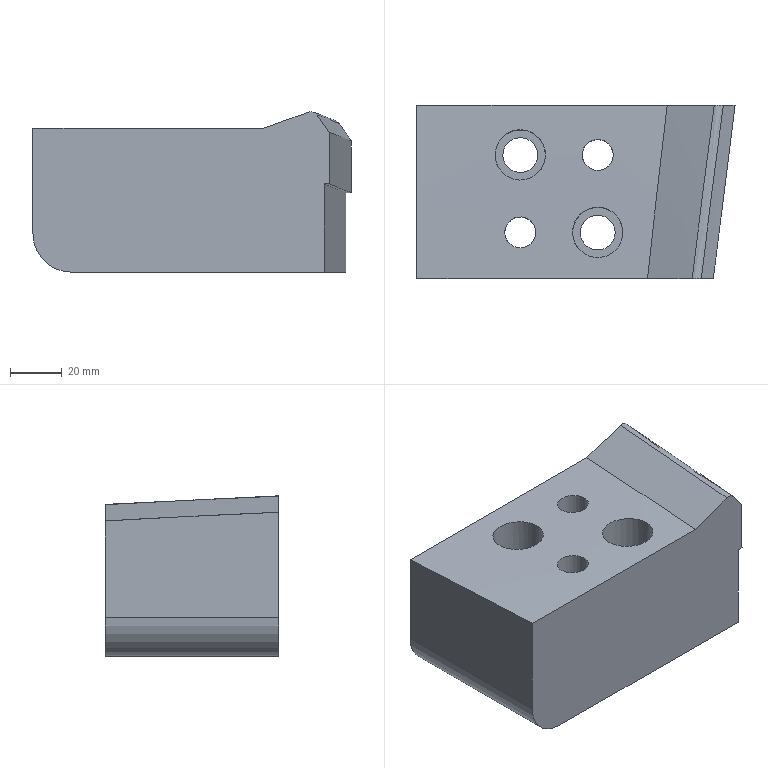Part | NX | features MAIN_BODY 2 | 1 solid | 20 faces | box 123.132 x 67 x 62.076 mm | volume 387142 mm3 | spline 7 | cylinder 7 | plane 6 | commonest cylinder face diameters 12 x2 13.5 x2 19.5 x2 30 x1
STEP:
#1=CARTESIAN_POINT('',(-841.75,399.358,-90.));
#2=VERTEX_POINT('',#1);
#3=CARTESIAN_POINT('',(-835.,399.358,-90.));
#4=DIRECTION('',(-0.000000341,-0.00000017,-1.));
#5=DIRECTION('',(-1.,0.,0.000000341));
#6=AXIS2_PLACEMENT_3D('',#3,#4,#5);
#7=CIRCLE('',#6,6.75);
#8=EDGE_CURVE('',#2,#2,#7,.F.);
#9=ORIENTED_EDGE('',*,*,#8,.T.);
#10=EDGE_LOOP('',(#9));
#11=FACE_BOUND('',#10,.T.);
#12=CARTESIAN_POINT('',(-841.,369.358,-90.));
#13=VERTEX_POINT('',#12);
#14=CARTESIAN_POINT('',(-835.,369.358,-90.));
#15=DIRECTION('',(-0.000000341,-0.00000017,-1.));
#16=DIRECTION('',(-1.,0.,0.000000341));
#17=AXIS2_PLACEMENT_3D('',#14,#15,#16);
#18=CIRCLE('',#17,6.);
#19=EDGE_CURVE('',#13,#13,#18,.F.);
#20=ORIENTED_EDGE('',*,*,#19,.T.);
#21=EDGE_LOOP('',(#20));
#22=FACE_BOUND('',#21,.T.);
#23=CARTESIAN_POINT('',(-811.75,369.358,-90.));
#24=VERTEX_POINT('',#23);
#25=CARTESIAN_POINT('',(-805.,369.358,-90.));
#26=DIRECTION('',(-0.000000341,-0.00000017,-1.));
#27=DIRECTION('',(-1.,0.,0.000000341));
#28=AXIS2_PLACEMENT_3D('',#25,#26,#27);
#29=CIRCLE('',#28,6.75);
#30=EDGE_CURVE('',#24,#24,#29,.F.);
#31=ORIENTED_EDGE('',*,*,#30,.T.);
#32=EDGE_LOOP('',(#31));
#33=FACE_BOUND('',#32,.T.);
#34=CARTESIAN_POINT('',(-811.,399.358,-90.));
#35=VERTEX_POINT('',#34);
#36=CARTESIAN_POINT('',(-805.,399.358,-90.));
#37=DIRECTION('',(-0.000000341,-0.00000017,-1.));
#38=DIRECTION('',(-1.,0.,0.000000341));
#39=AXIS2_PLACEMENT_3D('',#36,#37,#38);
#40=CIRCLE('',#39,6.);
#41=EDGE_CURVE('',#35,#35,#40,.F.);
#42=ORIENTED_EDGE('',*,*,#41,.T.);
#43=EDGE_LOOP('',(#42));
#44=FACE_BOUND('',#43,.T.);
#45=CARTESIAN_POINT('',(-860.,351.533,-90.));
#46=VERTEX_POINT('',#45);
#47=CARTESIAN_POINT('',(-762.297,351.533,-90.));
#48=VERTEX_POINT('',#47);
#49=CARTESIAN_POINT('',(-780.,351.533,-90.));
#50=DIRECTION('',(1.,0.000000011,-0.000000341));
#51=VECTOR('',#50,1000.);
#52=LINE('',#49,#51);
#53=EDGE_CURVE('',#46,#48,#52,.T.);
#54=ORIENTED_EDGE('',*,*,#53,.F.);
#55=CARTESIAN_POINT('',(-860.,418.533,-90.));
#56=VERTEX_POINT('',#55);
#57=CARTESIAN_POINT('',(-860.,1058.533,-90.));
#58=DIRECTION('',(-0.000000011,1.,-0.00000017));
#59=VECTOR('',#58,1000.);
#60=LINE('',#57,#59);
#61=EDGE_CURVE('',#46,#56,#60,.T.);
#62=ORIENTED_EDGE('',*,*,#61,.T.);
#63=CARTESIAN_POINT('',(-753.885,418.533,-90.));
#64=VERTEX_POINT('',#63);
#65=CARTESIAN_POINT('',(-780.,418.533,-90.));
#66=DIRECTION('',(1.,0.000000011,-0.000000341));
#67=VECTOR('',#66,1000.);
#68=LINE('',#65,#67);
#69=EDGE_CURVE('',#56,#64,#68,.T.);
#70=ORIENTED_EDGE('',*,*,#69,.T.);
#71=CARTESIAN_POINT('',(-753.885,418.533,-90.));
#72=CARTESIAN_POINT('',(-755.339,407.373,-90.));
#73=CARTESIAN_POINT('',(-758.303,385.059,-90.));
#74=CARTESIAN_POINT('',(-760.967,362.708,-90.));
#75=CARTESIAN_POINT('',(-762.297,351.533,-90.));
#76=B_SPLINE_CURVE_WITH_KNOTS('',3,(#71,#72,#73,#74,#75),.UNSPECIFIED.,.F.,.F.,(4,1,4),(0.,0.03376,0.06753),.UNSPECIFIED.);
#77=EDGE_CURVE('',#64,#48,#76,.T.);
#78=ORIENTED_EDGE('',*,*,#77,.T.);
#79=EDGE_LOOP('',(#54,#62,#70,#78));
#80=FACE_BOUND('',#79,.T.);
#81=CARTESIAN_POINT('',(-780.,1058.533,-90.));
#82=DIRECTION('',(-0.000000341,-0.00000017,-1.));
#83=DIRECTION('',(-0.000000011,1.,-0.00000017));
#84=AXIS2_PLACEMENT_3D('',#81,#82,#83);
#85=PLANE('',#84);
#86=ADVANCED_FACE('',(#11,#22,#33,#44,#80),#85,.T.);
#87=CARTESIAN_POINT('',(-751.868,418.533,-39.201));
#88=VERTEX_POINT('',#87);
#89=CARTESIAN_POINT('',(-756.435,418.533,-32.553));
#90=VERTEX_POINT('',#89);
#91=CARTESIAN_POINT('',(-751.868,418.533,-39.201));
#92=CARTESIAN_POINT('',(-753.39,418.533,-36.985));
#93=CARTESIAN_POINT('',(-754.912,418.533,-34.769));
#94=CARTESIAN_POINT('',(-756.435,418.533,-32.553));
#95=B_SPLINE_CURVE_WITH_KNOTS('',3,(#91,#92,#93,#94),.UNSPECIFIED.,.F.,.F.,(4,4),(0.,0.008065),.UNSPECIFIED.);
#96=EDGE_CURVE('',#88,#90,#95,.T.);
#97=ORIENTED_EDGE('',*,*,#96,.F.);
#98=CARTESIAN_POINT('',(-751.868,418.533,-59.201));
#99=VERTEX_POINT('',#98);
#100=CARTESIAN_POINT('',(-751.868,418.533,-39.201));
#101=CARTESIAN_POINT('',(-751.868,418.533,-45.868));
#102=CARTESIAN_POINT('',(-751.868,418.533,-52.535));
#103=CARTESIAN_POINT('',(-751.868,418.533,-59.201));
#104=B_SPLINE_CURVE_WITH_KNOTS('',3,(#100,#101,#102,#103),.UNSPECIFIED.,.F.,.F.,(4,4),(0.01625,0.03625),.UNSPECIFIED.);
#105=EDGE_CURVE('',#88,#99,#104,.T.);
#106=ORIENTED_EDGE('',*,*,#105,.T.);
#107=CARTESIAN_POINT('',(-753.885,418.533,-59.187));
#108=VERTEX_POINT('',#107);
#109=CARTESIAN_POINT('',(-753.885,418.533,-59.187));
#110=CARTESIAN_POINT('',(-753.213,418.533,-59.192));
#111=CARTESIAN_POINT('',(-752.541,418.533,-59.197));
#112=CARTESIAN_POINT('',(-751.868,418.533,-59.201));
#113=B_SPLINE_CURVE_WITH_KNOTS('',3,(#109,#110,#111,#112),.UNSPECIFIED.,.F.,.F.,(4,4),(0.,0.002017),.UNSPECIFIED.);
#114=EDGE_CURVE('',#108,#99,#113,.T.);
#115=ORIENTED_EDGE('',*,*,#114,.F.);
#116=CARTESIAN_POINT('',(-753.885,418.533,-59.187));
#117=CARTESIAN_POINT('',(-753.885,418.533,-69.458));
#118=CARTESIAN_POINT('',(-753.885,418.533,-79.729));
#119=CARTESIAN_POINT('',(-753.885,418.533,-90.));
#120=B_SPLINE_CURVE_WITH_KNOTS('',3,(#116,#117,#118,#119),.UNSPECIFIED.,.F.,.F.,(4,4),(-0.004527,0.02629),.UNSPECIFIED.);
#121=EDGE_CURVE('',#108,#64,#120,.T.);
#122=ORIENTED_EDGE('',*,*,#121,.T.);
#123=ORIENTED_EDGE('',*,*,#69,.F.);
#124=CARTESIAN_POINT('',(-875.,418.533,-75.));
#125=VERTEX_POINT('',#124);
#126=CARTESIAN_POINT('',(-860.,418.533,-75.));
#127=DIRECTION('',(-0.000000011,1.,-0.00000017));
#128=DIRECTION('',(0.,0.00000017,1.));
#129=AXIS2_PLACEMENT_3D('',#126,#127,#128);
#130=CIRCLE('',#129,15.);
#131=EDGE_CURVE('',#56,#125,#130,.T.);
#132=ORIENTED_EDGE('',*,*,#131,.T.);
#133=CARTESIAN_POINT('',(-875.,418.533,-37.652));
#134=VERTEX_POINT('',#133);
#135=CARTESIAN_POINT('',(-875.,418.533,-90.));
#136=DIRECTION('',(-0.000000341,-0.00000017,-1.));
#137=VECTOR('',#136,1000.);
#138=LINE('',#135,#137);
#139=EDGE_CURVE('',#125,#134,#138,.F.);
#140=ORIENTED_EDGE('',*,*,#139,.T.);
#141=CARTESIAN_POINT('',(-778.148,418.533,-37.652));
#142=VERTEX_POINT('',#141);
#143=CARTESIAN_POINT('',(-820.117,418.533,-37.652));
#144=DIRECTION('',(1.,0.000000011,-0.000000341));
#145=VECTOR('',#144,1000.);
#146=LINE('',#143,#145);
#147=EDGE_CURVE('',#134,#142,#146,.T.);
#148=ORIENTED_EDGE('',*,*,#147,.T.);
#149=CARTESIAN_POINT('',(-759.941,418.533,-31.393));
#150=VERTEX_POINT('',#149);
#151=CARTESIAN_POINT('',(-759.941,418.533,-31.393));
#152=CARTESIAN_POINT('',(-766.01,418.533,-33.479));
#153=CARTESIAN_POINT('',(-772.079,418.533,-35.565));
#154=CARTESIAN_POINT('',(-778.148,418.533,-37.652));
#155=B_SPLINE_CURVE_WITH_KNOTS('',3,(#151,#152,#153,#154),.UNSPECIFIED.,.F.,.F.,(4,4),(0.02556,0.04482),.UNSPECIFIED.);
#156=EDGE_CURVE('',#150,#142,#155,.T.);
#157=ORIENTED_EDGE('',*,*,#156,.F.);
#158=CARTESIAN_POINT('',(-756.435,418.533,-32.553));
#159=CARTESIAN_POINT('',(-757.19,418.533,-31.454));
#160=CARTESIAN_POINT('',(-758.679,418.533,-30.959));
#161=CARTESIAN_POINT('',(-759.941,418.533,-31.393));
#162=B_SPLINE_CURVE_WITH_KNOTS('',3,(#158,#159,#160,#161),.UNSPECIFIED.,.F.,.F.,(4,4),(0.,0.003944),.UNSPECIFIED.);
#163=EDGE_CURVE('',#90,#150,#162,.T.);
#164=ORIENTED_EDGE('',*,*,#163,.F.);
#165=EDGE_LOOP('',(#97,#106,#115,#122,#123,#132,#140,#148,#157,#164));
#166=FACE_BOUND('',#165,.T.);
#167=CARTESIAN_POINT('',(-840.,418.533,-90.));
#168=DIRECTION('',(-0.000000011,1.,-0.00000017));
#169=DIRECTION('',(0.000000341,0.00000017,1.));
#170=AXIS2_PLACEMENT_3D('',#167,#168,#169);
#171=PLANE('',#170);
#172=ADVANCED_FACE('',(#166),#171,.T.);
#173=CARTESIAN_POINT('',(-760.283,351.533,-35.819));
#174=VERTEX_POINT('',#173);
#175=CARTESIAN_POINT('',(-760.283,351.533,-55.819));
#176=VERTEX_POINT('',#175);
#177=CARTESIAN_POINT('',(-760.283,351.533,-35.819));
#178=CARTESIAN_POINT('',(-760.283,351.533,-42.486));
#179=CARTESIAN_POINT('',(-760.283,351.533,-49.152));
#180=CARTESIAN_POINT('',(-760.283,351.533,-55.819));
#181=B_SPLINE_CURVE_WITH_KNOTS('',3,(#177,#178,#179,#180),.UNSPECIFIED.,.F.,.F.,(4,4),(0.009058,0.02906),.UNSPECIFIED.);
#182=EDGE_CURVE('',#174,#176,#181,.T.);
#183=ORIENTED_EDGE('',*,*,#182,.T.);
#184=CARTESIAN_POINT('',(-751.868,418.533,-59.201));
#185=CARTESIAN_POINT('',(-753.322,407.375,-58.596));
#186=CARTESIAN_POINT('',(-756.286,385.067,-57.354));
#187=CARTESIAN_POINT('',(-758.953,362.711,-56.325));
#188=CARTESIAN_POINT('',(-760.283,351.533,-55.819));
#189=B_SPLINE_CURVE_WITH_KNOTS('',3,(#184,#185,#186,#187,#188),.UNSPECIFIED.,.F.,.F.,(4,1,4),(0.,0.03381,0.06761),.UNSPECIFIED.);
#190=EDGE_CURVE('',#99,#176,#189,.T.);
#191=ORIENTED_EDGE('',*,*,#190,.F.);
#192=ORIENTED_EDGE('',*,*,#105,.F.);
#193=CARTESIAN_POINT('',(-760.283,351.533,-35.819));
#194=CARTESIAN_POINT('',(-758.953,362.711,-36.325));
#195=CARTESIAN_POINT('',(-756.286,385.067,-37.354));
#196=CARTESIAN_POINT('',(-753.322,407.375,-38.596));
#197=CARTESIAN_POINT('',(-751.868,418.533,-39.201));
#198=B_SPLINE_CURVE_WITH_KNOTS('',3,(#193,#194,#195,#196,#197),.UNSPECIFIED.,.F.,.F.,(4,1,4),(0.,0.03381,0.06761),.UNSPECIFIED.);
#199=EDGE_CURVE('',#174,#88,#198,.T.);
#200=ORIENTED_EDGE('',*,*,#199,.F.);
#201=EDGE_LOOP('',(#183,#191,#192,#200));
#202=FACE_BOUND('',#201,.T.);
#203=CARTESIAN_POINT('',(-760.331,351.13,-55.941));
#204=CARTESIAN_POINT('',(-760.331,351.13,-35.657));
#205=CARTESIAN_POINT('',(-758.993,362.375,-56.467));
#206=CARTESIAN_POINT('',(-758.993,362.375,-36.183));
#207=CARTESIAN_POINT('',(-756.313,384.864,-57.522));
#208=CARTESIAN_POINT('',(-756.313,384.864,-37.238));
#209=CARTESIAN_POINT('',(-753.331,407.307,-58.731));
#210=CARTESIAN_POINT('',(-753.331,407.307,-38.447));
#211=CARTESIAN_POINT('',(-751.868,418.533,-59.322));
#212=CARTESIAN_POINT('',(-751.868,418.533,-39.037));
#213=B_SPLINE_SURFACE_WITH_KNOTS('',3,1,((#203,#204),(#205,#206),(#207,#208),(#209,#210),(#211,#212)),.SURF_OF_LINEAR_EXTRUSION.,.F.,.F.,.F.,(4,1,4),(2,2),(-0.3914,0.6746,1.741),(0.,1.),.UNSPECIFIED.);
#214=ADVANCED_FACE('',(#202),#213,.T.);
#215=ORIENTED_EDGE('',*,*,#139,.F.);
#216=CARTESIAN_POINT('',(-875.,351.533,-75.));
#217=VERTEX_POINT('',#216);
#218=CARTESIAN_POINT('',(-875.,739.25,-75.));
#219=DIRECTION('',(0.000000011,-1.,0.00000017));
#220=VECTOR('',#219,1000.);
#221=LINE('',#218,#220);
#222=EDGE_CURVE('',#125,#217,#221,.T.);
#223=ORIENTED_EDGE('',*,*,#222,.T.);
#224=CARTESIAN_POINT('',(-875.,351.533,-34.317));
#225=VERTEX_POINT('',#224);
#226=CARTESIAN_POINT('',(-875.,351.533,-90.));
#227=DIRECTION('',(-0.000000341,-0.00000017,-1.));
#228=VECTOR('',#227,1000.);
#229=LINE('',#226,#228);
#230=EDGE_CURVE('',#217,#225,#229,.F.);
#231=ORIENTED_EDGE('',*,*,#230,.T.);
#232=CARTESIAN_POINT('',(-875.,351.533,-34.317));
#233=CARTESIAN_POINT('',(-875.,373.874,-35.265));
#234=CARTESIAN_POINT('',(-875.,396.208,-36.367));
#235=CARTESIAN_POINT('',(-875.,418.533,-37.652));
#236=B_SPLINE_CURVE_WITH_KNOTS('',3,(#232,#233,#234,#235),.UNSPECIFIED.,.F.,.F.,(4,4),(0.277,0.3441),.UNSPECIFIED.);
#237=EDGE_CURVE('',#134,#225,#236,.F.);
#238=ORIENTED_EDGE('',*,*,#237,.F.);
#239=EDGE_LOOP('',(#215,#223,#231,#238));
#240=FACE_BOUND('',#239,.T.);
#241=CARTESIAN_POINT('',(-875.,739.25,-90.));
#242=DIRECTION('',(-1.,-0.000000011,0.000000341));
#243=DIRECTION('',(-0.000000341,-0.00000017,-1.));
#244=AXIS2_PLACEMENT_3D('',#241,#242,#243);
#245=PLANE('',#244);
#246=ADVANCED_FACE('',(#240),#245,.T.);
#247=CARTESIAN_POINT('',(-802.615,378.812,-35.56));
#248=VERTEX_POINT('',#247);
#249=CARTESIAN_POINT('',(-810.554,378.63,-35.551));
#250=CARTESIAN_POINT('',(-802.353,379.838,-35.61));
#251=CARTESIAN_POINT('',(-795.722,374.891,-35.371));
#252=CARTESIAN_POINT('',(-794.523,366.727,-34.987));
#253=CARTESIAN_POINT('',(-799.45,360.085,-34.688));
#254=CARTESIAN_POINT('',(-807.643,358.881,-34.635));
#255=CARTESIAN_POINT('',(-814.27,363.813,-34.854));
#256=CARTESIAN_POINT('',(-815.479,371.987,-35.232));
#257=CARTESIAN_POINT('',(-810.554,378.63,-35.551));
#258=CARTESIAN_POINT('',(-802.353,379.838,-35.61));
#259=CARTESIAN_POINT('',(-795.722,374.891,-35.371));
#260=B_SPLINE_CURVE_WITH_KNOTS('',3,(#249,#250,#251,#252,#253,#254,#255,#256,#257,#258,#259),.UNSPECIFIED.,.T.,.F.,(1,1,1,1,1,1,1,1,1,1,1,1,1,1,1),(-0.02287,-0.01525,-0.007624,0.,0.007624,0.01525,0.02287,0.0305,0.03812,0.04574,0.05337,0.06099,0.06862,0.07624,0.08386),.UNSPECIFIED.);
#261=EDGE_CURVE('',#248,#248,#260,.T.);
#262=ORIENTED_EDGE('',*,*,#261,.T.);
#263=EDGE_LOOP('',(#262));
#264=FACE_BOUND('',#263,.T.);
#265=CARTESIAN_POINT('',(-806.104,405.256,-36.91));
#266=VERTEX_POINT('',#265);
#267=CARTESIAN_POINT('',(-810.492,403.108,-36.793));
#268=CARTESIAN_POINT('',(-806.223,405.897,-36.944));
#269=CARTESIAN_POINT('',(-801.239,404.841,-36.887));
#270=CARTESIAN_POINT('',(-798.467,400.584,-36.658));
#271=CARTESIAN_POINT('',(-799.51,395.607,-36.398));
#272=CARTESIAN_POINT('',(-803.775,392.823,-36.256));
#273=CARTESIAN_POINT('',(-808.753,393.871,-36.309));
#274=CARTESIAN_POINT('',(-811.534,398.131,-36.529));
#275=CARTESIAN_POINT('',(-810.492,403.108,-36.793));
#276=CARTESIAN_POINT('',(-806.223,405.897,-36.944));
#277=CARTESIAN_POINT('',(-801.239,404.841,-36.887));
#278=B_SPLINE_CURVE_WITH_KNOTS('',3,(#267,#268,#269,#270,#271,#272,#273,#274,#275,#276,#277),.UNSPECIFIED.,.T.,.F.,(1,1,1,1,1,1,1,1,1,1,1,1,1,1,1),(-0.01408,-0.009385,-0.004692,0.,0.004692,0.009385,0.01408,0.01877,0.02346,0.02815,0.03285,0.03754,0.04223,0.04692,0.05162),.UNSPECIFIED.);
#279=EDGE_CURVE('',#266,#266,#278,.T.);
#280=ORIENTED_EDGE('',*,*,#279,.T.);
#281=EDGE_LOOP('',(#280));
#282=FACE_BOUND('',#281,.T.);
#283=CARTESIAN_POINT('',(-785.768,351.533,-34.317));
#284=VERTEX_POINT('',#283);
#285=CARTESIAN_POINT('',(-823.992,351.533,-34.317));
#286=DIRECTION('',(1.,0.000000011,-0.000000341));
#287=VECTOR('',#286,1000.);
#288=LINE('',#285,#287);
#289=EDGE_CURVE('',#225,#284,#288,.T.);
#290=ORIENTED_EDGE('',*,*,#289,.T.);
#291=CARTESIAN_POINT('',(-778.148,418.533,-37.652));
#292=CARTESIAN_POINT('',(-780.817,396.223,-36.368));
#293=CARTESIAN_POINT('',(-783.364,373.889,-35.266));
#294=CARTESIAN_POINT('',(-785.768,351.533,-34.317));
#295=B_SPLINE_CURVE_WITH_KNOTS('',3,(#291,#292,#293,#294),.UNSPECIFIED.,.F.,.F.,(4,4),(0.1671,0.2344),.UNSPECIFIED.);
#296=EDGE_CURVE('',#142,#284,#295,.T.);
#297=ORIENTED_EDGE('',*,*,#296,.F.);
#298=ORIENTED_EDGE('',*,*,#147,.F.);
#299=ORIENTED_EDGE('',*,*,#237,.T.);
#300=EDGE_LOOP('',(#290,#297,#298,#299));
#301=FACE_BOUND('',#300,.T.);
#302=CARTESIAN_POINT('',(-837.117,374.973,-35.376));
#303=VERTEX_POINT('',#302);
#304=CARTESIAN_POINT('',(-841.061,372.092,-35.239));
#305=CARTESIAN_POINT('',(-837.346,375.582,-35.405));
#306=CARTESIAN_POINT('',(-832.255,375.414,-35.397));
#307=CARTESIAN_POINT('',(-828.781,371.706,-35.22));
#308=CARTESIAN_POINT('',(-828.94,366.622,-34.983));
#309=CARTESIAN_POINT('',(-832.652,363.137,-34.825));
#310=CARTESIAN_POINT('',(-837.736,363.299,-34.832));
#311=CARTESIAN_POINT('',(-841.22,367.009,-35.001));
#312=CARTESIAN_POINT('',(-841.061,372.092,-35.239));
#313=CARTESIAN_POINT('',(-837.346,375.582,-35.405));
#314=CARTESIAN_POINT('',(-832.255,375.414,-35.397));
#315=B_SPLINE_CURVE_WITH_KNOTS('',3,(#304,#305,#306,#307,#308,#309,#310,#311,#312,#313,#314),.UNSPECIFIED.,.T.,.F.,(1,1,1,1,1,1,1,1,1,1,1,1,1,1,1),(-0.01408,-0.009384,-0.004692,0.,0.004692,0.009384,0.01408,0.01877,0.02346,0.02815,0.03284,0.03753,0.04223,0.04692,0.05161),.UNSPECIFIED.);
#316=EDGE_CURVE('',#303,#303,#315,.T.);
#317=ORIENTED_EDGE('',*,*,#316,.T.);
#318=EDGE_LOOP('',(#317));
#319=FACE_BOUND('',#318,.T.);
#320=CARTESIAN_POINT('',(-844.701,400.333,-36.646));
#321=VERTEX_POINT('',#320);
#322=CARTESIAN_POINT('',(-843.364,392.516,-36.238));
#323=CARTESIAN_POINT('',(-845.751,400.44,-36.648));
#324=CARTESIAN_POINT('',(-841.839,407.721,-37.043));
#325=CARTESIAN_POINT('',(-833.927,410.11,-37.176));
#326=CARTESIAN_POINT('',(-826.634,406.198,-36.959));
#327=CARTESIAN_POINT('',(-824.252,398.282,-36.535));
#328=CARTESIAN_POINT('',(-828.148,391.005,-36.162));
#329=CARTESIAN_POINT('',(-836.069,388.604,-36.043));
#330=CARTESIAN_POINT('',(-843.364,392.516,-36.238));
#331=CARTESIAN_POINT('',(-845.751,400.44,-36.648));
#332=CARTESIAN_POINT('',(-841.839,407.721,-37.043));
#333=B_SPLINE_CURVE_WITH_KNOTS('',3,(#322,#323,#324,#325,#326,#327,#328,#329,#330,#331,#332),.UNSPECIFIED.,.T.,.F.,(1,1,1,1,1,1,1,1,1,1,1,1,1,1,1),(-0.02288,-0.01525,-0.007625,0.,0.007625,0.01525,0.02288,0.0305,0.03813,0.04575,0.05338,0.061,0.06863,0.07625,0.08388),.UNSPECIFIED.);
#334=EDGE_CURVE('',#321,#321,#333,.T.);
#335=ORIENTED_EDGE('',*,*,#334,.T.);
#336=EDGE_LOOP('',(#335));
#337=FACE_BOUND('',#336,.T.);
#338=CARTESIAN_POINT('',(-875.586,418.533,-37.652));
#339=CARTESIAN_POINT('',(-776.779,418.533,-37.652));
#340=CARTESIAN_POINT('',(-877.041,407.36,-37.009));
#341=CARTESIAN_POINT('',(-778.234,407.36,-37.009));
#342=CARTESIAN_POINT('',(-880.005,385.084,-35.832));
#343=CARTESIAN_POINT('',(-781.198,385.084,-35.832));
#344=CARTESIAN_POINT('',(-882.657,362.711,-34.791));
#345=CARTESIAN_POINT('',(-783.85,362.711,-34.791));
#346=CARTESIAN_POINT('',(-883.99,351.533,-34.317));
#347=CARTESIAN_POINT('',(-785.183,351.533,-34.317));
#348=B_SPLINE_SURFACE_WITH_KNOTS('',3,1,((#338,#339),(#340,#341),(#342,#343),(#344,#345),(#346,#347)),.SURF_OF_LINEAR_EXTRUSION.,.F.,.F.,.F.,(4,1,4),(2,2),(-0.00601,0.4948,0.9956),(0.,1.),.UNSPECIFIED.);
#349=ADVANCED_FACE('',(#264,#282,#301,#319,#337),#348,.T.);
#350=CARTESIAN_POINT('',(-768.455,351.533,-28.093));
#351=VERTEX_POINT('',#350);
#352=CARTESIAN_POINT('',(-785.768,351.533,-34.317));
#353=CARTESIAN_POINT('',(-779.997,351.533,-32.242));
#354=CARTESIAN_POINT('',(-774.226,351.533,-30.167));
#355=CARTESIAN_POINT('',(-768.455,351.533,-28.093));
#356=B_SPLINE_CURVE_WITH_KNOTS('',3,(#352,#353,#354,#355),.UNSPECIFIED.,.F.,.F.,(4,4),(0.07252,0.09092),.UNSPECIFIED.);
#357=EDGE_CURVE('',#351,#284,#356,.F.);
#358=ORIENTED_EDGE('',*,*,#357,.T.);
#359=ORIENTED_EDGE('',*,*,#289,.F.);
#360=ORIENTED_EDGE('',*,*,#230,.F.);
#361=CARTESIAN_POINT('',(-860.,351.533,-75.));
#362=DIRECTION('',(-0.000000011,1.,-0.00000017));
#363=DIRECTION('',(0.,0.00000017,1.));
#364=AXIS2_PLACEMENT_3D('',#361,#362,#363);
#365=CIRCLE('',#364,15.);
#366=EDGE_CURVE('',#217,#46,#365,.F.);
#367=ORIENTED_EDGE('',*,*,#366,.T.);
#368=ORIENTED_EDGE('',*,*,#53,.T.);
#369=CARTESIAN_POINT('',(-762.297,351.533,-55.808));
#370=VERTEX_POINT('',#369);
#371=CARTESIAN_POINT('',(-762.297,351.533,-55.808));
#372=CARTESIAN_POINT('',(-762.297,351.533,-67.206));
#373=CARTESIAN_POINT('',(-762.297,351.533,-78.603));
#374=CARTESIAN_POINT('',(-762.297,351.533,-90.));
#375=B_SPLINE_CURVE_WITH_KNOTS('',3,(#371,#372,#373,#374),.UNSPECIFIED.,.F.,.F.,(4,4),(-0.01041,0.02379),.UNSPECIFIED.);
#376=EDGE_CURVE('',#370,#48,#375,.T.);
#377=ORIENTED_EDGE('',*,*,#376,.F.);
#378=CARTESIAN_POINT('',(-760.283,351.533,-55.819));
#379=CARTESIAN_POINT('',(-760.955,351.533,-55.816));
#380=CARTESIAN_POINT('',(-761.626,351.533,-55.812));
#381=CARTESIAN_POINT('',(-762.297,351.533,-55.808));
#382=B_SPLINE_CURVE_WITH_KNOTS('',3,(#378,#379,#380,#381),.UNSPECIFIED.,.F.,.F.,(4,4),(0.,0.002014),.UNSPECIFIED.);
#383=EDGE_CURVE('',#176,#370,#382,.T.);
#384=ORIENTED_EDGE('',*,*,#383,.F.);
#385=ORIENTED_EDGE('',*,*,#182,.F.);
#386=CARTESIAN_POINT('',(-764.943,351.533,-29.203));
#387=VERTEX_POINT('',#386);
#388=CARTESIAN_POINT('',(-764.943,351.533,-29.203));
#389=CARTESIAN_POINT('',(-763.39,351.533,-31.408));
#390=CARTESIAN_POINT('',(-761.836,351.533,-33.614));
#391=CARTESIAN_POINT('',(-760.283,351.533,-35.819));
#392=B_SPLINE_CURVE_WITH_KNOTS('',3,(#388,#389,#390,#391),.UNSPECIFIED.,.F.,.F.,(4,4),(0.007518,0.01561),.UNSPECIFIED.);
#393=EDGE_CURVE('',#387,#174,#392,.T.);
#394=ORIENTED_EDGE('',*,*,#393,.F.);
#395=CARTESIAN_POINT('',(-768.455,351.533,-28.093));
#396=CARTESIAN_POINT('',(-767.203,351.533,-27.643));
#397=CARTESIAN_POINT('',(-765.71,351.533,-28.115));
#398=CARTESIAN_POINT('',(-764.943,351.533,-29.203));
#399=B_SPLINE_CURVE_WITH_KNOTS('',3,(#395,#396,#397,#398),.UNSPECIFIED.,.F.,.F.,(4,4),(0.,0.003935),.UNSPECIFIED.);
#400=EDGE_CURVE('',#351,#387,#399,.T.);
#401=ORIENTED_EDGE('',*,*,#400,.F.);
#402=EDGE_LOOP('',(#358,#359,#360,#367,#368,#377,#384,#385,#394,#401));
#403=FACE_BOUND('',#402,.T.);
#404=CARTESIAN_POINT('',(-840.,351.533,-90.));
#405=DIRECTION('',(-0.000000011,1.,-0.00000017));
#406=DIRECTION('',(0.000000341,0.00000017,1.));
#407=AXIS2_PLACEMENT_3D('',#404,#405,#406);
#408=PLANE('',#407);
#409=ADVANCED_FACE('',(#403),#408,.F.);
#410=CARTESIAN_POINT('',(-844.75,399.358,-80.));
#411=VERTEX_POINT('',#410);
#412=CARTESIAN_POINT('',(-835.,399.358,-80.));
#413=DIRECTION('',(-0.000000341,-0.00000017,-1.));
#414=DIRECTION('',(-1.,0.,0.000000341));
#415=AXIS2_PLACEMENT_3D('',#412,#413,#414);
#416=CIRCLE('',#415,9.75);
#417=EDGE_CURVE('',#411,#411,#416,.F.);
#418=ORIENTED_EDGE('',*,*,#417,.F.);
#419=EDGE_LOOP('',(#418));
#420=FACE_BOUND('',#419,.T.);
#421=ORIENTED_EDGE('',*,*,#334,.F.);
#422=EDGE_LOOP('',(#421));
#423=FACE_BOUND('',#422,.T.);
#424=CARTESIAN_POINT('',(-835.,399.358,-70.));
#425=DIRECTION('',(0.000000341,0.00000017,1.));
#426=DIRECTION('',(0.000000011,-1.,0.00000017));
#427=AXIS2_PLACEMENT_3D('',#424,#425,#426);
#428=CYLINDRICAL_SURFACE('',#427,9.75);
#429=ADVANCED_FACE('',(#420,#423),#428,.F.);
#430=CARTESIAN_POINT('',(-841.75,399.358,-80.));
#431=VERTEX_POINT('',#430);
#432=CARTESIAN_POINT('',(-835.,399.358,-80.));
#433=DIRECTION('',(-0.000000341,-0.00000017,-1.));
#434=DIRECTION('',(-1.,0.,0.000000341));
#435=AXIS2_PLACEMENT_3D('',#432,#433,#434);
#436=CIRCLE('',#435,6.75);
#437=EDGE_CURVE('',#431,#431,#436,.F.);
#438=ORIENTED_EDGE('',*,*,#437,.T.);
#439=EDGE_LOOP('',(#438));
#440=FACE_BOUND('',#439,.T.);
#441=ORIENTED_EDGE('',*,*,#8,.F.);
#442=EDGE_LOOP('',(#441));
#443=FACE_BOUND('',#442,.T.);
#444=CARTESIAN_POINT('',(-835.,399.358,-90.));
#445=DIRECTION('',(0.000000341,0.00000017,1.));
#446=DIRECTION('',(0.000000011,-1.,0.00000017));
#447=AXIS2_PLACEMENT_3D('',#444,#445,#446);
#448=CYLINDRICAL_SURFACE('',#447,6.75);
#449=ADVANCED_FACE('',(#440,#443),#448,.F.);
#450=ORIENTED_EDGE('',*,*,#437,.F.);
#451=EDGE_LOOP('',(#450));
#452=FACE_BOUND('',#451,.T.);
#453=ORIENTED_EDGE('',*,*,#417,.T.);
#454=EDGE_LOOP('',(#453));
#455=FACE_BOUND('',#454,.T.);
#456=CARTESIAN_POINT('',(-835.,399.358,-80.));
#457=DIRECTION('',(-0.000000341,-0.00000017,-1.));
#458=DIRECTION('',(-0.000000011,1.,-0.00000017));
#459=AXIS2_PLACEMENT_3D('',#456,#457,#458);
#460=PLANE('',#459);
#461=ADVANCED_FACE('',(#452,#455),#460,.F.);
#462=ORIENTED_EDGE('',*,*,#19,.F.);
#463=EDGE_LOOP('',(#462));
#464=FACE_BOUND('',#463,.T.);
#465=ORIENTED_EDGE('',*,*,#316,.F.);
#466=EDGE_LOOP('',(#465));
#467=FACE_BOUND('',#466,.T.);
#468=CARTESIAN_POINT('',(-835.,369.358,-90.));
#469=DIRECTION('',(0.000000341,0.00000017,1.));
#470=DIRECTION('',(0.000000011,-1.,0.00000017));
#471=AXIS2_PLACEMENT_3D('',#468,#469,#470);
#472=CYLINDRICAL_SURFACE('',#471,6.);
#473=ADVANCED_FACE('',(#464,#467),#472,.F.);
#474=CARTESIAN_POINT('',(-814.75,369.358,-80.));
#475=VERTEX_POINT('',#474);
#476=CARTESIAN_POINT('',(-805.,369.358,-80.));
#477=DIRECTION('',(-0.000000341,-0.00000017,-1.));
#478=DIRECTION('',(-1.,0.,0.000000341));
#479=AXIS2_PLACEMENT_3D('',#476,#477,#478);
#480=CIRCLE('',#479,9.75);
#481=EDGE_CURVE('',#475,#475,#480,.F.);
#482=ORIENTED_EDGE('',*,*,#481,.F.);
#483=EDGE_LOOP('',(#482));
#484=FACE_BOUND('',#483,.T.);
#485=ORIENTED_EDGE('',*,*,#261,.F.);
#486=EDGE_LOOP('',(#485));
#487=FACE_BOUND('',#486,.T.);
#488=CARTESIAN_POINT('',(-805.,369.358,-70.));
#489=DIRECTION('',(0.000000341,0.00000017,1.));
#490=DIRECTION('',(0.000000011,-1.,0.00000017));
#491=AXIS2_PLACEMENT_3D('',#488,#489,#490);
#492=CYLINDRICAL_SURFACE('',#491,9.75);
#493=ADVANCED_FACE('',(#484,#487),#492,.F.);
#494=CARTESIAN_POINT('',(-811.75,369.358,-80.));
#495=VERTEX_POINT('',#494);
#496=CARTESIAN_POINT('',(-805.,369.358,-80.));
#497=DIRECTION('',(-0.000000341,-0.00000017,-1.));
#498=DIRECTION('',(-1.,0.,0.000000341));
#499=AXIS2_PLACEMENT_3D('',#496,#497,#498);
#500=CIRCLE('',#499,6.75);
#501=EDGE_CURVE('',#495,#495,#500,.F.);
#502=ORIENTED_EDGE('',*,*,#501,.T.);
#503=EDGE_LOOP('',(#502));
#504=FACE_BOUND('',#503,.T.);
#505=ORIENTED_EDGE('',*,*,#30,.F.);
#506=EDGE_LOOP('',(#505));
#507=FACE_BOUND('',#506,.T.);
#508=CARTESIAN_POINT('',(-805.,369.358,-90.));
#509=DIRECTION('',(0.000000341,0.00000017,1.));
#510=DIRECTION('',(0.000000011,-1.,0.00000017));
#511=AXIS2_PLACEMENT_3D('',#508,#509,#510);
#512=CYLINDRICAL_SURFACE('',#511,6.75);
#513=ADVANCED_FACE('',(#504,#507),#512,.F.);
#514=ORIENTED_EDGE('',*,*,#501,.F.);
#515=EDGE_LOOP('',(#514));
#516=FACE_BOUND('',#515,.T.);
#517=ORIENTED_EDGE('',*,*,#481,.T.);
#518=EDGE_LOOP('',(#517));
#519=FACE_BOUND('',#518,.T.);
#520=CARTESIAN_POINT('',(-805.,369.358,-80.));
#521=DIRECTION('',(-0.000000341,-0.00000017,-1.));
#522=DIRECTION('',(-0.000000011,1.,-0.00000017));
#523=AXIS2_PLACEMENT_3D('',#520,#521,#522);
#524=PLANE('',#523);
#525=ADVANCED_FACE('',(#516,#519),#524,.F.);
#526=ORIENTED_EDGE('',*,*,#41,.F.);
#527=EDGE_LOOP('',(#526));
#528=FACE_BOUND('',#527,.T.);
#529=ORIENTED_EDGE('',*,*,#279,.F.);
#530=EDGE_LOOP('',(#529));
#531=FACE_BOUND('',#530,.T.);
#532=CARTESIAN_POINT('',(-805.,399.358,-90.));
#533=DIRECTION('',(0.000000341,0.00000017,1.));
#534=DIRECTION('',(0.000000011,-1.,0.00000017));
#535=AXIS2_PLACEMENT_3D('',#532,#533,#534);
#536=CYLINDRICAL_SURFACE('',#535,6.);
#537=ADVANCED_FACE('',(#528,#531),#536,.F.);
#538=ORIENTED_EDGE('',*,*,#114,.T.);
#539=ORIENTED_EDGE('',*,*,#190,.T.);
#540=ORIENTED_EDGE('',*,*,#383,.T.);
#541=CARTESIAN_POINT('',(-753.885,418.533,-59.187));
#542=CARTESIAN_POINT('',(-755.339,407.375,-58.581));
#543=CARTESIAN_POINT('',(-758.302,385.067,-57.341));
#544=CARTESIAN_POINT('',(-760.967,362.711,-56.314));
#545=CARTESIAN_POINT('',(-762.297,351.533,-55.808));
#546=B_SPLINE_CURVE_WITH_KNOTS('',3,(#541,#542,#543,#544,#545),.UNSPECIFIED.,.F.,.F.,(4,1,4),(0.,0.03381,0.06761),.UNSPECIFIED.);
#547=EDGE_CURVE('',#108,#370,#546,.T.);
#548=ORIENTED_EDGE('',*,*,#547,.F.);
#549=EDGE_LOOP('',(#538,#539,#540,#548));
#550=FACE_BOUND('',#549,.T.);
#551=CARTESIAN_POINT('',(-751.849,418.53,-59.201));
#552=CARTESIAN_POINT('',(-753.303,407.372,-58.596));
#553=CARTESIAN_POINT('',(-754.778,396.218,-57.973));
#554=CARTESIAN_POINT('',(-757.606,373.887,-56.841));
#555=CARTESIAN_POINT('',(-758.933,362.709,-56.325));
#556=CARTESIAN_POINT('',(-760.264,351.53,-55.819));
#557=CARTESIAN_POINT('',(-760.289,351.317,-55.809));
#558=CARTESIAN_POINT('',(-760.314,351.104,-55.8));
#559=CARTESIAN_POINT('',(-760.34,350.89,-55.79));
#560=CARTESIAN_POINT('',(-753.869,418.793,-59.201));
#561=CARTESIAN_POINT('',(-755.323,407.637,-58.596));
#562=CARTESIAN_POINT('',(-756.799,396.482,-57.973));
#563=CARTESIAN_POINT('',(-759.629,374.135,-56.841));
#564=CARTESIAN_POINT('',(-760.957,362.946,-56.325));
#565=CARTESIAN_POINT('',(-762.287,351.771,-55.819));
#566=CARTESIAN_POINT('',(-762.312,351.558,-55.809));
#567=CARTESIAN_POINT('',(-762.338,351.344,-55.8));
#568=CARTESIAN_POINT('',(-762.363,351.131,-55.79));
#569=B_SPLINE_SURFACE_WITH_KNOTS('',1,3,((#551,#552,#553,#554,#555,#556,#557,#558,#559),(#560,#561,#562,#563,#564,#565,#566,#567,#568)),.RULED_SURF.,.F.,.F.,.F.,(2,2),(4,2,3,4),(0.498,0.7018),(0.,0.5,1.,1.01),.UNSPECIFIED.);
#570=ADVANCED_FACE('',(#550),#569,.F.);
#571=ORIENTED_EDGE('',*,*,#547,.T.);
#572=ORIENTED_EDGE('',*,*,#376,.T.);
#573=ORIENTED_EDGE('',*,*,#77,.F.);
#574=ORIENTED_EDGE('',*,*,#121,.F.);
#575=EDGE_LOOP('',(#571,#572,#573,#574));
#576=FACE_BOUND('',#575,.T.);
#577=CARTESIAN_POINT('',(-762.345,351.13,-90.186));
#578=CARTESIAN_POINT('',(-762.345,351.13,-55.559));
#579=CARTESIAN_POINT('',(-760.999,362.438,-90.716));
#580=CARTESIAN_POINT('',(-760.999,362.438,-56.089));
#581=CARTESIAN_POINT('',(-758.303,385.072,-91.776));
#582=CARTESIAN_POINT('',(-758.303,385.072,-57.149));
#583=CARTESIAN_POINT('',(-755.304,407.645,-92.992));
#584=CARTESIAN_POINT('',(-755.304,407.645,-58.365));
#585=CARTESIAN_POINT('',(-753.833,418.934,-93.586));
#586=CARTESIAN_POINT('',(-753.833,418.934,-58.959));
#587=B_SPLINE_SURFACE_WITH_KNOTS('',3,1,((#577,#578),(#579,#580),(#581,#582),(#583,#584),(#585,#586)),.SURF_OF_LINEAR_EXTRUSION.,.F.,.F.,.F.,(4,1,4),(2,2),(-0.3989,0.6732,1.745),(0.,1.),.UNSPECIFIED.);
#588=ADVANCED_FACE('',(#576),#587,.T.);
#589=ORIENTED_EDGE('',*,*,#131,.F.);
#590=ORIENTED_EDGE('',*,*,#61,.F.);
#591=ORIENTED_EDGE('',*,*,#366,.F.);
#592=ORIENTED_EDGE('',*,*,#222,.F.);
#593=EDGE_LOOP('',(#589,#590,#591,#592));
#594=FACE_BOUND('',#593,.T.);
#595=CARTESIAN_POINT('',(-860.,739.25,-75.));
#596=DIRECTION('',(0.000000011,-1.,0.00000017));
#597=DIRECTION('',(-0.000000341,-0.00000017,-1.));
#598=AXIS2_PLACEMENT_3D('',#595,#596,#597);
#599=CYLINDRICAL_SURFACE('',#598,15.);
#600=ADVANCED_FACE('',(#594),#599,.T.);
#601=ORIENTED_EDGE('',*,*,#156,.T.);
#602=ORIENTED_EDGE('',*,*,#296,.T.);
#603=ORIENTED_EDGE('',*,*,#357,.F.);
#604=CARTESIAN_POINT('',(-759.941,418.533,-31.393));
#605=CARTESIAN_POINT('',(-762.945,396.23,-30.121));
#606=CARTESIAN_POINT('',(-765.792,373.895,-29.032));
#607=CARTESIAN_POINT('',(-768.455,351.533,-28.093));
#608=B_SPLINE_CURVE_WITH_KNOTS('',3,(#604,#605,#606,#607),.UNSPECIFIED.,.F.,.F.,(4,4),(0.,0.06762),.UNSPECIFIED.);
#609=EDGE_CURVE('',#150,#351,#608,.T.);
#610=ORIENTED_EDGE('',*,*,#609,.F.);
#611=EDGE_LOOP('',(#601,#602,#603,#610));
#612=FACE_BOUND('',#611,.T.);
#613=CARTESIAN_POINT('',(-786.227,351.139,-34.45));
#614=CARTESIAN_POINT('',(-780.194,350.971,-32.266));
#615=CARTESIAN_POINT('',(-774.162,350.804,-30.083));
#616=CARTESIAN_POINT('',(-768.129,350.637,-27.9));
#617=CARTESIAN_POINT('',(-783.783,373.942,-35.412));
#618=CARTESIAN_POINT('',(-777.723,373.788,-33.248));
#619=CARTESIAN_POINT('',(-771.662,373.634,-31.084));
#620=CARTESIAN_POINT('',(-765.602,373.48,-28.921));
#621=CARTESIAN_POINT('',(-781.094,396.652,-36.506));
#622=CARTESIAN_POINT('',(-775.002,396.517,-34.364));
#623=CARTESIAN_POINT('',(-768.91,396.381,-32.222));
#624=CARTESIAN_POINT('',(-762.818,396.245,-30.08));
#625=CARTESIAN_POINT('',(-778.161,419.269,-37.729));
#626=CARTESIAN_POINT('',(-772.033,419.158,-35.612));
#627=CARTESIAN_POINT('',(-765.905,419.046,-33.495));
#628=CARTESIAN_POINT('',(-759.778,418.934,-31.379));
#629=B_SPLINE_SURFACE_WITH_KNOTS('',3,3,((#613,#614,#615,#616),(#617,#618,#619,#620),(#621,#622,#623,#624),(#625,#626,#627,#628)),.UNSPECIFIED.,.F.,.F.,.F.,(4,4),(4,4),(0.6097,0.7303),(-0.6399,-0.1096),.UNSPECIFIED.);
#630=ADVANCED_FACE('',(#612),#629,.F.);
#631=ORIENTED_EDGE('',*,*,#393,.T.);
#632=ORIENTED_EDGE('',*,*,#199,.T.);
#633=ORIENTED_EDGE('',*,*,#96,.T.);
#634=CARTESIAN_POINT('',(-764.943,351.533,-29.203));
#635=CARTESIAN_POINT('',(-762.283,373.896,-30.158));
#636=CARTESIAN_POINT('',(-759.436,396.23,-31.263));
#637=CARTESIAN_POINT('',(-756.435,418.533,-32.553));
#638=B_SPLINE_CURVE_WITH_KNOTS('',3,(#634,#635,#636,#637),.UNSPECIFIED.,.F.,.F.,(4,4),(0.,0.06762),.UNSPECIFIED.);
#639=EDGE_CURVE('',#387,#90,#638,.T.);
#640=ORIENTED_EDGE('',*,*,#639,.F.);
#641=EDGE_LOOP('',(#631,#632,#633,#640));
#642=FACE_BOUND('',#641,.T.);
#643=CARTESIAN_POINT('',(-740.786,416.476,-55.625));
#644=CARTESIAN_POINT('',(-754.076,419.45,-35.862));
#645=CARTESIAN_POINT('',(-760.511,420.89,-26.291));
#646=CARTESIAN_POINT('',(-741.502,410.76,-55.318));
#647=CARTESIAN_POINT('',(-754.82,413.687,-35.566));
#648=CARTESIAN_POINT('',(-761.268,415.105,-26.002));
#649=CARTESIAN_POINT('',(-742.219,405.044,-55.01));
#650=CARTESIAN_POINT('',(-755.564,407.925,-35.271));
#651=CARTESIAN_POINT('',(-762.026,409.321,-25.713));
#652=CARTESIAN_POINT('',(-742.935,399.328,-54.703));
#653=CARTESIAN_POINT('',(-756.308,402.163,-34.976));
#654=CARTESIAN_POINT('',(-762.783,403.536,-25.424));
#655=CARTESIAN_POINT('',(-743.651,393.612,-54.395));
#656=CARTESIAN_POINT('',(-757.052,396.401,-34.681));
#657=CARTESIAN_POINT('',(-763.54,397.751,-25.135));
#658=CARTESIAN_POINT('',(-744.368,387.896,-54.088));
#659=CARTESIAN_POINT('',(-757.796,390.639,-34.386));
#660=CARTESIAN_POINT('',(-764.298,391.967,-24.846));
#661=CARTESIAN_POINT('',(-744.908,383.586,-53.856));
#662=CARTESIAN_POINT('',(-758.357,386.294,-34.163));
#663=CARTESIAN_POINT('',(-764.869,387.605,-24.628));
#664=CARTESIAN_POINT('',(-745.44,379.274,-53.629));
#665=CARTESIAN_POINT('',(-758.909,381.948,-33.945));
#666=CARTESIAN_POINT('',(-765.431,383.243,-24.414));
#667=CARTESIAN_POINT('',(-745.964,374.962,-53.405));
#668=CARTESIAN_POINT('',(-759.454,377.601,-33.731));
#669=CARTESIAN_POINT('',(-765.985,378.879,-24.204));
#670=CARTESIAN_POINT('',(-746.481,370.648,-53.187));
#671=CARTESIAN_POINT('',(-759.99,373.253,-33.521));
#672=CARTESIAN_POINT('',(-766.531,374.514,-23.999));
#673=CARTESIAN_POINT('',(-746.989,366.332,-52.972));
#674=CARTESIAN_POINT('',(-760.517,368.904,-33.316));
#675=CARTESIAN_POINT('',(-767.068,370.149,-23.798));
#676=CARTESIAN_POINT('',(-747.432,362.573,-52.785));
#677=CARTESIAN_POINT('',(-760.977,365.115,-33.136));
#678=CARTESIAN_POINT('',(-767.536,366.346,-23.622));
#679=CARTESIAN_POINT('',(-747.874,358.814,-52.598));
#680=CARTESIAN_POINT('',(-761.437,361.326,-32.957));
#681=CARTESIAN_POINT('',(-768.004,362.543,-23.447));
#682=CARTESIAN_POINT('',(-748.317,355.055,-52.411));
#683=CARTESIAN_POINT('',(-761.896,357.537,-32.778));
#684=CARTESIAN_POINT('',(-768.472,358.74,-23.271));
#685=CARTESIAN_POINT('',(-748.76,351.295,-52.224));
#686=CARTESIAN_POINT('',(-762.356,353.749,-32.599));
#687=CARTESIAN_POINT('',(-768.94,354.937,-23.096));
#688=CARTESIAN_POINT('',(-749.203,347.536,-52.037));
#689=CARTESIAN_POINT('',(-762.816,349.96,-32.419));
#690=CARTESIAN_POINT('',(-769.408,351.134,-22.92));
#691=B_SPLINE_SURFACE_WITH_KNOTS('',5,1,((#643,#644,#645),(#646,#647,#648),(#649,#650,#651),(#652,#653,#654),(#655,#656,#657),(#658,#659,#660),(#661,#662,#663),(#664,#665,#666),(#667,#668,#669),(#670,#671,#672),(#673,#674,#675),(#676,#677,#678),(#679,#680,#681),(#682,#683,#684),(#685,#686,#687),(#688,#689,#690)),.RULED_SURF.,.F.,.F.,.F.,(6,5,5,6),(2,1,2),(-1.326,0.,1.,1.871),(0.,1.,1.484),.PIECEWISE_BEZIER_KNOTS.);
#692=ADVANCED_FACE('',(#642),#691,.F.);
#693=ORIENTED_EDGE('',*,*,#163,.T.);
#694=ORIENTED_EDGE('',*,*,#609,.T.);
#695=ORIENTED_EDGE('',*,*,#400,.T.);
#696=ORIENTED_EDGE('',*,*,#639,.T.);
#697=EDGE_LOOP('',(#693,#694,#695,#696));
#698=FACE_BOUND('',#697,.T.);
#699=CARTESIAN_POINT('',(-765.046,350.671,-29.166));
#700=CARTESIAN_POINT('',(-766.352,350.905,-27.284));
#701=CARTESIAN_POINT('',(-768.503,351.127,-28.076));
#702=CARTESIAN_POINT('',(-762.338,373.461,-30.135));
#703=CARTESIAN_POINT('',(-763.634,373.712,-28.247));
#704=CARTESIAN_POINT('',(-765.789,373.935,-29.032));
#705=CARTESIAN_POINT('',(-759.44,396.209,-31.26));
#706=CARTESIAN_POINT('',(-760.728,396.472,-29.367));
#707=CARTESIAN_POINT('',(-762.883,396.715,-30.143));
#708=CARTESIAN_POINT('',(-756.38,418.937,-32.576));
#709=CARTESIAN_POINT('',(-757.657,419.217,-30.679));
#710=CARTESIAN_POINT('',(-759.815,419.463,-31.446));
#711=(BOUNDED_SURFACE()B_SPLINE_SURFACE(3,2,((#699,#700,#701),(#702,#703,#704),(#705,#706,#707),(#708,#709,#710)),.UNSPECIFIED.,.F.,.F.,.F.)B_SPLINE_SURFACE_WITH_KNOTS((4,4),(3,3),(0.07434,0.1433),(0.,1.),.PIECEWISE_BEZIER_KNOTS.)GEOMETRIC_REPRESENTATION_ITEM()RATIONAL_B_SPLINE_SURFACE(((1.,0.7932,1.),(1.,0.7931,1.),(1.,0.7931,1.),(1.,0.7931,1.)))REPRESENTATION_ITEM('')SURFACE());
#712=ADVANCED_FACE('',(#698),#711,.T.);
#713=CLOSED_SHELL('',(#86,#172,#214,#246,#349,#409,#429,#449,#461,#473,#493,#513,#525,#537,#570,#588,#600,#630,#692,#712));
#714=MANIFOLD_SOLID_BREP('',#713);
#715=(LENGTH_UNIT()NAMED_UNIT(*)SI_UNIT(.MILLI.,.METRE.));
#716=UNCERTAINTY_MEASURE_WITH_UNIT(LENGTH_MEASURE(0.0508),#715,'','');
#717=(NAMED_UNIT(*)PLANE_ANGLE_UNIT()SI_UNIT($,.RADIAN.));
#718=(NAMED_UNIT(*)SI_UNIT($,.STERADIAN.)SOLID_ANGLE_UNIT());
#719=(GEOMETRIC_REPRESENTATION_CONTEXT(3)GLOBAL_UNCERTAINTY_ASSIGNED_CONTEXT((#716))GLOBAL_UNIT_ASSIGNED_CONTEXT((#715,#717,#718))REPRESENTATION_CONTEXT('',''));
#720=ADVANCED_BREP_SHAPE_REPRESENTATION('',(#714),#719);